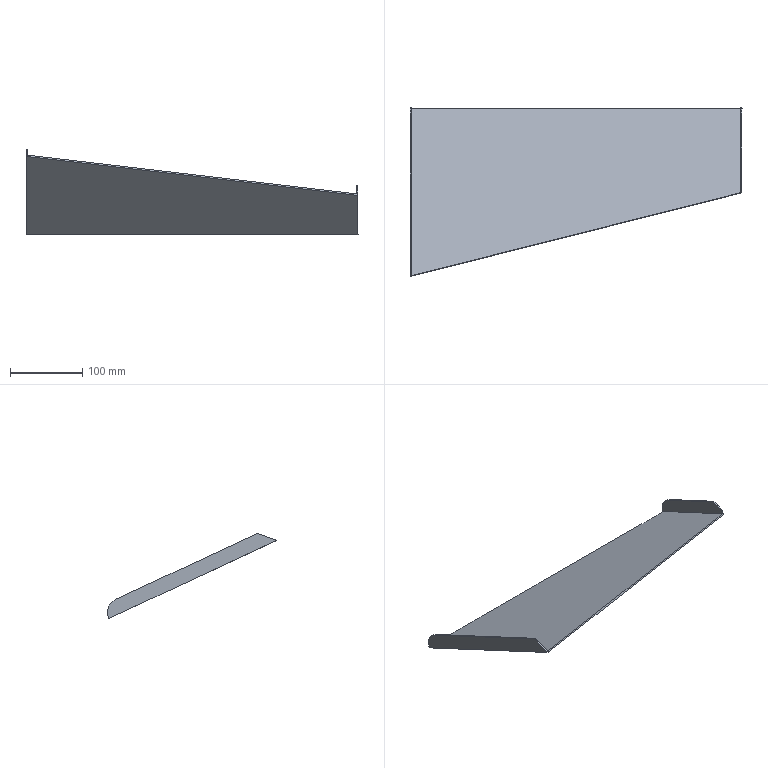Part | NX | features solid 2 | 1 solid | 16 faces | box 459.183 x 234.003 x 117.917 mm | volume 189236 mm3 | plane 13 | cylinder 2 | spline 1 | commonest cylinder face diameters 40 x2
STEP:
#1=CARTESIAN_POINT('',(244.183,710.326,-255.572));
#2=VERTEX_POINT('',#1);
#3=CARTESIAN_POINT('',(244.183,622.552,-214.642));
#4=VERTEX_POINT('',#3);
#5=CARTESIAN_POINT('',(244.183,728.452,-264.024));
#6=DIRECTION('',(0.,-0.9063,0.4226));
#7=VECTOR('',#6,1000.);
#8=LINE('',#5,#7);
#9=EDGE_CURVE('',#2,#4,#8,.T.);
#10=ORIENTED_EDGE('',*,*,#9,.F.);
#11=CARTESIAN_POINT('',(242.183,710.326,-255.572));
#12=VERTEX_POINT('',#11);
#13=CARTESIAN_POINT('',(214.183,710.326,-255.572));
#14=DIRECTION('',(-1.,0.,0.));
#15=VECTOR('',#14,1000.);
#16=LINE('',#13,#15);
#17=EDGE_CURVE('',#2,#12,#16,.T.);
#18=ORIENTED_EDGE('',*,*,#17,.T.);
#19=CARTESIAN_POINT('',(242.183,622.552,-214.642));
#20=VERTEX_POINT('',#19);
#21=CARTESIAN_POINT('',(242.183,728.452,-264.024));
#22=DIRECTION('',(0.,-0.9063,0.4226));
#23=VECTOR('',#22,1000.);
#24=LINE('',#21,#23);
#25=EDGE_CURVE('',#12,#20,#24,.T.);
#26=ORIENTED_EDGE('',*,*,#25,.T.);
#27=CARTESIAN_POINT('',(214.183,622.552,-214.642));
#28=DIRECTION('',(1.,0.,0.));
#29=VECTOR('',#28,1000.);
#30=LINE('',#27,#29);
#31=EDGE_CURVE('',#20,#4,#30,.T.);
#32=ORIENTED_EDGE('',*,*,#31,.T.);
#33=EDGE_LOOP('',(#10,#18,#26,#32));
#34=FACE_BOUND('',#33,.T.);
#35=CARTESIAN_POINT('',(214.183,728.452,-264.024));
#36=DIRECTION('',(0.,-0.4226,-0.9063));
#37=DIRECTION('',(0.,-0.9063,0.4226));
#38=AXIS2_PLACEMENT_3D('',#35,#36,#37);
#39=PLANE('',#38);
#40=ADVANCED_FACE('',(#34),#39,.F.);
#41=CARTESIAN_POINT('',(242.183,720.,-279.943));
#42=VERTEX_POINT('',#41);
#43=CARTESIAN_POINT('',(242.183,603.874,-225.793));
#44=VERTEX_POINT('',#43);
#45=CARTESIAN_POINT('',(242.183,417.055,-138.678));
#46=DIRECTION('',(0.,-0.9063,0.4226));
#47=VECTOR('',#46,1000.);
#48=LINE('',#45,#47);
#49=EDGE_CURVE('',#42,#44,#48,.T.);
#50=ORIENTED_EDGE('',*,*,#49,.T.);
#51=CARTESIAN_POINT('',(242.183,606.319,-220.55));
#52=VERTEX_POINT('',#51);
#53=CARTESIAN_POINT('',(242.183,606.319,-220.55));
#54=DIRECTION('',(0.,-0.4226,-0.9063));
#55=VECTOR('',#54,1000.);
#56=LINE('',#53,#55);
#57=EDGE_CURVE('',#44,#52,#56,.F.);
#58=ORIENTED_EDGE('',*,*,#57,.T.);
#59=CARTESIAN_POINT('',(242.183,686.904,-191.22));
#60=DIRECTION('',(0.,0.9397,0.342));
#61=VECTOR('',#60,1000.);
#62=LINE('',#59,#61);
#63=EDGE_CURVE('',#52,#20,#62,.T.);
#64=ORIENTED_EDGE('',*,*,#63,.T.);
#65=ORIENTED_EDGE('',*,*,#25,.F.);
#66=CARTESIAN_POINT('',(242.183,720.,-282.15));
#67=VERTEX_POINT('',#66);
#68=CARTESIAN_POINT('',(242.183,701.874,-273.698));
#69=DIRECTION('',(-1.,0.,0.));
#70=DIRECTION('',(0.,-1.,0.));
#71=AXIS2_PLACEMENT_3D('',#68,#69,#70);
#72=CIRCLE('',#71,20.);
#73=EDGE_CURVE('',#12,#67,#72,.T.);
#74=ORIENTED_EDGE('',*,*,#73,.T.);
#75=CARTESIAN_POINT('',(242.183,720.,-430.));
#76=DIRECTION('',(0.,0.,-1.));
#77=VECTOR('',#76,1000.);
#78=LINE('',#75,#77);
#79=EDGE_CURVE('',#42,#67,#78,.T.);
#80=ORIENTED_EDGE('',*,*,#79,.F.);
#81=EDGE_LOOP('',(#50,#58,#64,#65,#74,#80));
#82=FACE_BOUND('',#81,.T.);
#83=CARTESIAN_POINT('',(242.183,720.,-282.15));
#84=DIRECTION('',(-1.,0.,0.));
#85=DIRECTION('',(0.,-1.,0.));
#86=AXIS2_PLACEMENT_3D('',#83,#84,#85);
#87=PLANE('',#86);
#88=ADVANCED_FACE('',(#82),#87,.T.);
#89=ORIENTED_EDGE('',*,*,#63,.F.);
#90=CARTESIAN_POINT('',(244.183,607.058,-220.281));
#91=VERTEX_POINT('',#90);
#92=CARTESIAN_POINT('',(244.183,607.058,-220.281));
#93=CARTESIAN_POINT('',(243.516,606.812,-220.371));
#94=CARTESIAN_POINT('',(242.85,606.566,-220.461));
#95=CARTESIAN_POINT('',(242.183,606.319,-220.55));
#96=B_SPLINE_CURVE_WITH_KNOTS('',3,(#92,#93,#94,#95),.UNSPECIFIED.,.F.,.F.,(4,4),(0.1738,0.176),.UNSPECIFIED.);
#97=EDGE_CURVE('',#52,#91,#96,.F.);
#98=ORIENTED_EDGE('',*,*,#97,.T.);
#99=CARTESIAN_POINT('',(244.183,570.633,-233.539));
#100=DIRECTION('',(0.,-0.9397,-0.342));
#101=VECTOR('',#100,1000.);
#102=LINE('',#99,#101);
#103=EDGE_CURVE('',#4,#91,#102,.T.);
#104=ORIENTED_EDGE('',*,*,#103,.F.);
#105=ORIENTED_EDGE('',*,*,#31,.F.);
#106=EDGE_LOOP('',(#89,#98,#104,#105));
#107=FACE_BOUND('',#106,.T.);
#108=CARTESIAN_POINT('',(214.183,595.974,-224.316));
#109=DIRECTION('',(0.,-0.342,0.9397));
#110=DIRECTION('',(0.,-0.9397,-0.342));
#111=AXIS2_PLACEMENT_3D('',#108,#109,#110);
#112=PLANE('',#111);
#113=ADVANCED_FACE('',(#107),#112,.T.);
#114=CARTESIAN_POINT('',(244.183,603.533,-227.841));
#115=VERTEX_POINT('',#114);
#116=CARTESIAN_POINT('',(244.183,603.956,-226.934));
#117=DIRECTION('',(0.,-0.4226,-0.9063));
#118=VECTOR('',#117,1000.);
#119=LINE('',#116,#118);
#120=EDGE_CURVE('',#91,#115,#119,.T.);
#121=ORIENTED_EDGE('',*,*,#120,.T.);
#122=CARTESIAN_POINT('',(244.183,720.,-282.15));
#123=VERTEX_POINT('',#122);
#124=CARTESIAN_POINT('',(244.183,559.597,-207.353));
#125=DIRECTION('',(0.,-0.9063,0.4226));
#126=VECTOR('',#125,1000.);
#127=LINE('',#124,#126);
#128=EDGE_CURVE('',#123,#115,#127,.T.);
#129=ORIENTED_EDGE('',*,*,#128,.F.);
#130=CARTESIAN_POINT('',(244.183,701.874,-273.698));
#131=DIRECTION('',(1.,0.,0.));
#132=DIRECTION('',(0.,1.,0.));
#133=AXIS2_PLACEMENT_3D('',#130,#131,#132);
#134=CIRCLE('',#133,20.);
#135=EDGE_CURVE('',#123,#2,#134,.T.);
#136=ORIENTED_EDGE('',*,*,#135,.T.);
#137=ORIENTED_EDGE('',*,*,#9,.T.);
#138=ORIENTED_EDGE('',*,*,#103,.T.);
#139=EDGE_LOOP('',(#121,#129,#136,#137,#138));
#140=FACE_BOUND('',#139,.T.);
#141=CARTESIAN_POINT('',(244.183,560.442,-205.54));
#142=DIRECTION('',(1.,0.,0.));
#143=DIRECTION('',(0.,1.,0.));
#144=AXIS2_PLACEMENT_3D('',#141,#142,#143);
#145=PLANE('',#144);
#146=ADVANCED_FACE('',(#140),#145,.T.);
#147=ORIENTED_EDGE('',*,*,#135,.F.);
#148=CARTESIAN_POINT('',(188.564,720.,-282.15));
#149=DIRECTION('',(-1.,0.,0.));
#150=VECTOR('',#149,1000.);
#151=LINE('',#148,#150);
#152=EDGE_CURVE('',#123,#67,#151,.T.);
#153=ORIENTED_EDGE('',*,*,#152,.T.);
#154=ORIENTED_EDGE('',*,*,#73,.F.);
#155=ORIENTED_EDGE('',*,*,#17,.F.);
#156=EDGE_LOOP('',(#147,#153,#154,#155));
#157=FACE_BOUND('',#156,.T.);
#158=CARTESIAN_POINT('',(214.183,701.874,-273.698));
#159=DIRECTION('',(-1.,0.,0.));
#160=DIRECTION('',(0.,-1.,0.));
#161=AXIS2_PLACEMENT_3D('',#158,#159,#160);
#162=CYLINDRICAL_SURFACE('',#161,20.);
#163=ADVANCED_FACE('',(#157),#162,.T.);
#164=CARTESIAN_POINT('',(-213.,488.372,-174.14));
#165=VERTEX_POINT('',#164);
#166=CARTESIAN_POINT('',(-213.,488.372,-174.14));
#167=CARTESIAN_POINT('',(-174.889,497.929,-178.597));
#168=CARTESIAN_POINT('',(-98.706,517.168,-187.568));
#169=CARTESIAN_POINT('',(53.68,555.581,-205.48));
#170=CARTESIAN_POINT('',(167.988,584.333,-218.888));
#171=CARTESIAN_POINT('',(244.183,603.533,-227.841));
#172=B_SPLINE_CURVE_WITH_KNOTS('',3,(#166,#167,#168,#169,#170,#171),.UNSPECIFIED.,.F.,.F.,(4,1,1,4),(0.,0.1186,0.2373,0.4745),.UNSPECIFIED.);
#173=EDGE_CURVE('',#165,#115,#172,.T.);
#174=ORIENTED_EDGE('',*,*,#173,.F.);
#175=CARTESIAN_POINT('',(-213.,487.871,-173.907));
#176=VERTEX_POINT('',#175);
#177=CARTESIAN_POINT('',(-213.,487.871,-173.907));
#178=DIRECTION('',(0.,0.9063,-0.4226));
#179=VECTOR('',#178,1000.);
#180=LINE('',#177,#179);
#181=EDGE_CURVE('',#176,#165,#180,.T.);
#182=ORIENTED_EDGE('',*,*,#181,.F.);
#183=CARTESIAN_POINT('',(-215.,487.871,-173.907));
#184=VERTEX_POINT('',#183);
#185=CARTESIAN_POINT('',(-215.,487.871,-173.907));
#186=DIRECTION('',(1.,0.,0.));
#187=VECTOR('',#186,1000.);
#188=LINE('',#185,#187);
#189=EDGE_CURVE('',#184,#176,#188,.T.);
#190=ORIENTED_EDGE('',*,*,#189,.F.);
#191=CARTESIAN_POINT('',(-215.,720.,-282.15));
#192=VERTEX_POINT('',#191);
#193=CARTESIAN_POINT('',(-215.,416.21,-140.491));
#194=DIRECTION('',(0.,0.9063,-0.4226));
#195=VECTOR('',#194,1000.);
#196=LINE('',#193,#195);
#197=EDGE_CURVE('',#184,#192,#196,.T.);
#198=ORIENTED_EDGE('',*,*,#197,.T.);
#199=CARTESIAN_POINT('',(-213.,720.,-282.15));
#200=VERTEX_POINT('',#199);
#201=CARTESIAN_POINT('',(-215.,720.,-282.15));
#202=DIRECTION('',(1.,0.,0.));
#203=VECTOR('',#202,1000.);
#204=LINE('',#201,#203);
#205=EDGE_CURVE('',#192,#200,#204,.T.);
#206=ORIENTED_EDGE('',*,*,#205,.T.);
#207=CARTESIAN_POINT('',(188.564,720.,-282.15));
#208=DIRECTION('',(-1.,0.,0.));
#209=VECTOR('',#208,1000.);
#210=LINE('',#207,#209);
#211=EDGE_CURVE('',#67,#200,#210,.T.);
#212=ORIENTED_EDGE('',*,*,#211,.F.);
#213=ORIENTED_EDGE('',*,*,#152,.F.);
#214=ORIENTED_EDGE('',*,*,#128,.T.);
#215=EDGE_LOOP('',(#174,#182,#190,#198,#206,#212,#213,#214));
#216=FACE_BOUND('',#215,.T.);
#217=CARTESIAN_POINT('',(-353.018,416.21,-140.491));
#218=DIRECTION('',(0.,0.4226,0.9063));
#219=DIRECTION('',(1.,0.,0.));
#220=AXIS2_PLACEMENT_3D('',#217,#218,#219);
#221=PLANE('',#220);
#222=ADVANCED_FACE('',(#216),#221,.F.);
#223=CARTESIAN_POINT('',(221.376,598.631,-223.348));
#224=VERTEX_POINT('',#223);
#225=CARTESIAN_POINT('',(-677.72,244.443,-58.187));
#226=CARTESIAN_POINT('',(-660.306,267.421,-68.902));
#227=CARTESIAN_POINT('',(-639.328,288.979,-78.955));
#228=CARTESIAN_POINT('',(-618.744,310.134,-88.819));
#229=CARTESIAN_POINT('',(-595.443,329.078,-97.653));
#230=CARTESIAN_POINT('',(-550.727,365.432,-114.606));
#231=CARTESIAN_POINT('',(-494.661,394.945,-128.368));
#232=CARTESIAN_POINT('',(-442.667,422.315,-141.131));
#233=CARTESIAN_POINT('',(-382.139,443.144,-150.843));
#234=CARTESIAN_POINT('',(-352.965,453.184,-155.525));
#235=CARTESIAN_POINT('',(-323.451,461.202,-159.264));
#236=CARTESIAN_POINT('',(-311.851,464.353,-160.733));
#237=CARTESIAN_POINT('',(-289.398,470.048,-163.389));
#238=CARTESIAN_POINT('',(-278.105,472.912,-164.724));
#239=CARTESIAN_POINT('',(-263.795,476.502,-166.398));
#240=CARTESIAN_POINT('',(-257.293,478.133,-167.159));
#241=CARTESIAN_POINT('',(-233.907,483.982,-169.886));
#242=CARTESIAN_POINT('',(-218.807,487.759,-171.647));
#243=CARTESIAN_POINT('',(-204.022,491.47,-173.378));
#244=CARTESIAN_POINT('',(-178.964,497.761,-176.312));
#245=CARTESIAN_POINT('',(-144.274,506.511,-180.392));
#246=CARTESIAN_POINT('',(-27.735,535.905,-194.099));
#247=CARTESIAN_POINT('',(-24.798,536.645,-194.444));
#248=CARTESIAN_POINT('',(13.703,546.346,-198.967));
#249=CARTESIAN_POINT('',(94.693,566.731,-208.473));
#250=CARTESIAN_POINT('',(173.185,586.488,-217.686));
#251=CARTESIAN_POINT('',(214.183,596.819,-222.503));
#252=CARTESIAN_POINT('',(229.183,600.599,-224.266));
#253=CARTESIAN_POINT('',(244.183,604.378,-226.028));
#254=B_SPLINE_CURVE_WITH_KNOTS('',2,(#225,#226,#227,#228,#229,#230,#231,#232,#233,#234,#235,#236,#237,#238,#239,#240,#241,#242,#243,#244,#245,#246,#247,#248,#249,#250,#251,#252,#253),.UNSPECIFIED.,.F.,.F.,(3,2,2,2,2,2,2,2,2,2,2,2,2,2,3),(0.,0.0625,0.125,0.25,0.375,0.4375,0.4732,0.5,0.5312,0.5625,0.625,0.75,0.875,1.,1.046),.PIECEWISE_BEZIER_KNOTS.);
#255=EDGE_CURVE('',#224,#44,#254,.T.);
#256=ORIENTED_EDGE('',*,*,#255,.F.);
#257=CARTESIAN_POINT('',(-215.,488.716,-172.094));
#258=VERTEX_POINT('',#257);
#259=CARTESIAN_POINT('',(-215.,488.716,-172.094));
#260=CARTESIAN_POINT('',(-142.246,506.955,-180.599));
#261=CARTESIAN_POINT('',(3.163,543.756,-197.76));
#262=CARTESIAN_POINT('',(148.649,580.305,-214.803));
#263=CARTESIAN_POINT('',(221.376,598.631,-223.348));
#264=B_SPLINE_CURVE_WITH_KNOTS('',3,(#259,#260,#261,#262,#263),.UNSPECIFIED.,.F.,.F.,(4,1,4),(0.,0.2265,0.4529),.UNSPECIFIED.);
#265=EDGE_CURVE('',#258,#224,#264,.T.);
#266=ORIENTED_EDGE('',*,*,#265,.F.);
#267=CARTESIAN_POINT('',(-215.,488.294,-173.));
#268=DIRECTION('',(0.,-0.4226,-0.9063));
#269=VECTOR('',#268,1000.);
#270=LINE('',#267,#269);
#271=EDGE_CURVE('',#258,#184,#270,.T.);
#272=ORIENTED_EDGE('',*,*,#271,.T.);
#273=CARTESIAN_POINT('',(-213.,488.606,-173.639));
#274=VERTEX_POINT('',#273);
#275=CARTESIAN_POINT('',(-215.,487.871,-173.907));
#276=CARTESIAN_POINT('',(-214.333,488.116,-173.817));
#277=CARTESIAN_POINT('',(-213.667,488.361,-173.728));
#278=CARTESIAN_POINT('',(-213.,488.606,-173.639));
#279=B_SPLINE_CURVE_WITH_KNOTS('',3,(#275,#276,#277,#278),.UNSPECIFIED.,.F.,.F.,(4,4),(0.,0.002148),.UNSPECIFIED.);
#280=EDGE_CURVE('',#184,#274,#279,.T.);
#281=ORIENTED_EDGE('',*,*,#280,.T.);
#282=CARTESIAN_POINT('',(-213.,489.218,-172.328));
#283=DIRECTION('',(0.,-0.4226,-0.9063));
#284=VECTOR('',#283,1000.);
#285=LINE('',#282,#284);
#286=EDGE_CURVE('',#274,#165,#285,.T.);
#287=ORIENTED_EDGE('',*,*,#286,.T.);
#288=ORIENTED_EDGE('',*,*,#173,.T.);
#289=ORIENTED_EDGE('',*,*,#120,.F.);
#290=ORIENTED_EDGE('',*,*,#97,.F.);
#291=ORIENTED_EDGE('',*,*,#57,.F.);
#292=EDGE_LOOP('',(#256,#266,#272,#281,#287,#288,#289,#290,#291));
#293=FACE_BOUND('',#292,.T.);
#294=CARTESIAN_POINT('',(-215.,491.417,-166.302));
#295=CARTESIAN_POINT('',(-215.,487.871,-173.907));
#296=CARTESIAN_POINT('',(-213.771,491.725,-166.445));
#297=CARTESIAN_POINT('',(-213.771,488.179,-174.05));
#298=CARTESIAN_POINT('',(-211.321,492.34,-166.732));
#299=CARTESIAN_POINT('',(-211.321,488.794,-174.337));
#300=CARTESIAN_POINT('',(-208.246,493.111,-167.092));
#301=CARTESIAN_POINT('',(-208.246,489.565,-174.697));
#302=CARTESIAN_POINT('',(-205.832,493.717,-167.374));
#303=CARTESIAN_POINT('',(-205.832,490.171,-174.979));
#304=CARTESIAN_POINT('',(-203.913,494.199,-167.599));
#305=CARTESIAN_POINT('',(-203.913,490.653,-175.204));
#306=CARTESIAN_POINT('',(-202.454,494.565,-167.77));
#307=CARTESIAN_POINT('',(-202.454,491.019,-175.374));
#308=CARTESIAN_POINT('',(-200.317,495.102,-168.02));
#309=CARTESIAN_POINT('',(-200.317,491.555,-175.625));
#310=CARTESIAN_POINT('',(-197.658,495.77,-168.331));
#311=CARTESIAN_POINT('',(-197.658,492.223,-175.936));
#312=CARTESIAN_POINT('',(-193.272,496.872,-168.845));
#313=CARTESIAN_POINT('',(-193.272,493.326,-176.45));
#314=CARTESIAN_POINT('',(-187.616,498.294,-169.508));
#315=CARTESIAN_POINT('',(-187.616,494.747,-177.113));
#316=CARTESIAN_POINT('',(-180.53,500.076,-170.34));
#317=CARTESIAN_POINT('',(-180.53,496.53,-177.944));
#318=CARTESIAN_POINT('',(-173.151,501.934,-171.206));
#319=CARTESIAN_POINT('',(-173.151,498.388,-178.811));
#320=CARTESIAN_POINT('',(-166.755,503.545,-171.957));
#321=CARTESIAN_POINT('',(-166.755,499.999,-179.562));
#322=CARTESIAN_POINT('',(-161.492,504.871,-172.575));
#323=CARTESIAN_POINT('',(-161.492,501.325,-180.18));
#324=CARTESIAN_POINT('',(-157.47,505.885,-173.048));
#325=CARTESIAN_POINT('',(-157.47,502.338,-180.653));
#326=CARTESIAN_POINT('',(-154.057,506.745,-173.449));
#327=CARTESIAN_POINT('',(-154.057,503.199,-181.054));
#328=CARTESIAN_POINT('',(-151.291,507.442,-173.774));
#329=CARTESIAN_POINT('',(-151.291,503.896,-181.379));
#330=CARTESIAN_POINT('',(-149.195,507.971,-174.021));
#331=CARTESIAN_POINT('',(-149.195,504.425,-181.626));
#332=CARTESIAN_POINT('',(-147.441,508.413,-174.227));
#333=CARTESIAN_POINT('',(-147.441,504.867,-181.832));
#334=CARTESIAN_POINT('',(-146.012,508.774,-174.395));
#335=CARTESIAN_POINT('',(-146.012,505.227,-182.));
#336=CARTESIAN_POINT('',(-145.153,508.99,-174.496));
#337=CARTESIAN_POINT('',(-145.153,505.444,-182.101));
#338=CARTESIAN_POINT('',(-144.522,509.149,-174.57));
#339=CARTESIAN_POINT('',(-144.522,505.603,-182.175));
#340=CARTESIAN_POINT('',(-144.305,509.204,-174.596));
#341=CARTESIAN_POINT('',(-144.305,505.658,-182.201));
#342=CARTESIAN_POINT('',(-143.977,509.287,-174.635));
#343=CARTESIAN_POINT('',(-143.977,505.741,-182.239));
#344=CARTESIAN_POINT('',(-143.469,509.415,-174.694));
#345=CARTESIAN_POINT('',(-143.469,505.869,-182.299));
#346=CARTESIAN_POINT('',(-142.712,509.606,-174.783));
#347=CARTESIAN_POINT('',(-142.712,506.06,-182.388));
#348=CARTESIAN_POINT('',(-141.525,509.905,-174.923));
#349=CARTESIAN_POINT('',(-141.525,506.359,-182.528));
#350=CARTESIAN_POINT('',(-140.043,510.279,-175.097));
#351=CARTESIAN_POINT('',(-140.043,506.733,-182.702));
#352=CARTESIAN_POINT('',(-136.518,511.168,-175.512));
#353=CARTESIAN_POINT('',(-136.518,507.622,-183.117));
#354=CARTESIAN_POINT('',(-131.33,512.477,-176.122));
#355=CARTESIAN_POINT('',(-131.33,508.931,-183.727));
#356=CARTESIAN_POINT('',(-124.631,514.166,-176.91));
#357=CARTESIAN_POINT('',(-124.631,510.62,-184.515));
#358=CARTESIAN_POINT('',(-118.15,515.801,-177.672));
#359=CARTESIAN_POINT('',(-118.15,512.255,-185.277));
#360=CARTESIAN_POINT('',(-109.797,517.908,-178.655));
#361=CARTESIAN_POINT('',(-109.797,514.362,-186.259));
#362=CARTESIAN_POINT('',(-99.9,520.404,-179.819));
#363=CARTESIAN_POINT('',(-99.9,516.858,-187.424));
#364=CARTESIAN_POINT('',(-88.892,523.181,-181.113));
#365=CARTESIAN_POINT('',(-88.892,519.635,-188.718));
#366=CARTESIAN_POINT('',(-78.753,525.738,-182.306));
#367=CARTESIAN_POINT('',(-78.753,522.192,-189.911));
#368=CARTESIAN_POINT('',(-66.394,528.855,-183.759));
#369=CARTESIAN_POINT('',(-66.394,525.309,-191.364));
#370=CARTESIAN_POINT('',(-53.117,532.204,-185.321));
#371=CARTESIAN_POINT('',(-53.117,528.658,-192.926));
#372=CARTESIAN_POINT('',(-42.738,534.822,-186.542));
#373=CARTESIAN_POINT('',(-42.738,531.276,-194.147));
#374=CARTESIAN_POINT('',(-36.173,536.478,-187.314));
#375=CARTESIAN_POINT('',(-36.173,532.932,-194.919));
#376=CARTESIAN_POINT('',(-32.118,537.501,-187.791));
#377=CARTESIAN_POINT('',(-32.118,533.954,-195.396));
#378=CARTESIAN_POINT('',(-28.932,538.304,-188.165));
#379=CARTESIAN_POINT('',(-28.932,534.758,-195.77));
#380=CARTESIAN_POINT('',(-27.001,538.791,-188.392));
#381=CARTESIAN_POINT('',(-27.001,535.245,-195.997));
#382=CARTESIAN_POINT('',(-25.891,539.071,-188.523));
#383=CARTESIAN_POINT('',(-25.891,535.525,-196.128));
#384=CARTESIAN_POINT('',(-25.379,539.2,-188.583));
#385=CARTESIAN_POINT('',(-25.379,535.654,-196.188));
#386=CARTESIAN_POINT('',(-25.114,539.267,-188.614));
#387=CARTESIAN_POINT('',(-25.114,535.72,-196.219));
#388=CARTESIAN_POINT('',(-24.992,539.297,-188.629));
#389=CARTESIAN_POINT('',(-24.992,535.751,-196.234));
#390=CARTESIAN_POINT('',(-24.909,539.318,-188.638));
#391=CARTESIAN_POINT('',(-24.909,535.772,-196.243));
#392=CARTESIAN_POINT('',(-24.867,539.329,-188.643));
#393=CARTESIAN_POINT('',(-24.867,535.783,-196.248));
#394=CARTESIAN_POINT('',(-24.804,539.345,-188.651));
#395=CARTESIAN_POINT('',(-24.804,535.799,-196.256));
#396=CARTESIAN_POINT('',(-24.861,539.331,-188.644));
#397=CARTESIAN_POINT('',(-24.861,535.784,-196.249));
#398=CARTESIAN_POINT('',(-24.468,539.429,-188.69));
#399=CARTESIAN_POINT('',(-24.468,535.883,-196.295));
#400=CARTESIAN_POINT('',(-24.1,539.522,-188.734));
#401=CARTESIAN_POINT('',(-24.1,535.976,-196.338));
#402=CARTESIAN_POINT('',(-23.377,539.704,-188.818));
#403=CARTESIAN_POINT('',(-23.377,536.158,-196.423));
#404=CARTESIAN_POINT('',(-22.37,539.958,-188.937));
#405=CARTESIAN_POINT('',(-22.37,536.412,-196.542));
#406=CARTESIAN_POINT('',(-20.71,540.376,-189.132));
#407=CARTESIAN_POINT('',(-20.71,536.83,-196.737));
#408=CARTESIAN_POINT('',(-18.592,540.91,-189.381));
#409=CARTESIAN_POINT('',(-18.592,537.364,-196.985));
#410=CARTESIAN_POINT('',(-15.966,541.571,-189.689));
#411=CARTESIAN_POINT('',(-15.966,538.025,-197.294));
#412=CARTESIAN_POINT('',(-12.357,542.48,-190.113));
#413=CARTESIAN_POINT('',(-12.357,538.934,-197.718));
#414=CARTESIAN_POINT('',(-7.643,543.668,-190.667));
#415=CARTESIAN_POINT('',(-7.643,540.122,-198.272));
#416=CARTESIAN_POINT('',(-1.661,545.175,-191.369));
#417=CARTESIAN_POINT('',(-1.661,541.628,-198.974));
#418=CARTESIAN_POINT('',(4.647,546.763,-192.11));
#419=CARTESIAN_POINT('',(4.647,543.217,-199.715));
#420=CARTESIAN_POINT('',(13.49,548.99,-193.148));
#421=CARTESIAN_POINT('',(13.49,545.444,-200.753));
#422=CARTESIAN_POINT('',(25.356,551.978,-194.542));
#423=CARTESIAN_POINT('',(25.356,548.432,-202.146));
#424=CARTESIAN_POINT('',(40.897,555.89,-196.366));
#425=CARTESIAN_POINT('',(40.897,552.344,-203.971));
#426=CARTESIAN_POINT('',(54.93,559.423,-198.013));
#427=CARTESIAN_POINT('',(54.93,555.877,-205.618));
#428=CARTESIAN_POINT('',(66.808,562.413,-199.408));
#429=CARTESIAN_POINT('',(66.808,558.867,-207.013));
#430=CARTESIAN_POINT('',(76.04,564.737,-200.491));
#431=CARTESIAN_POINT('',(76.04,561.191,-208.096));
#432=CARTESIAN_POINT('',(84.008,566.743,-201.427));
#433=CARTESIAN_POINT('',(84.008,563.197,-209.031));
#434=CARTESIAN_POINT('',(90.536,568.386,-202.193));
#435=CARTESIAN_POINT('',(90.536,564.84,-209.798));
#436=CARTESIAN_POINT('',(97.206,570.065,-202.976));
#437=CARTESIAN_POINT('',(97.206,566.519,-210.581));
#438=CARTESIAN_POINT('',(105.077,572.046,-203.9));
#439=CARTESIAN_POINT('',(105.077,568.5,-211.504));
#440=CARTESIAN_POINT('',(117.449,575.16,-205.352));
#441=CARTESIAN_POINT('',(117.449,571.614,-212.957));
#442=CARTESIAN_POINT('',(132.141,578.859,-207.076));
#443=CARTESIAN_POINT('',(132.141,575.312,-214.681));
#444=CARTESIAN_POINT('',(148.648,583.014,-209.014));
#445=CARTESIAN_POINT('',(148.648,579.468,-216.619));
#446=CARTESIAN_POINT('',(164.001,586.88,-210.817));
#447=CARTESIAN_POINT('',(164.001,583.334,-218.422));
#448=CARTESIAN_POINT('',(178.208,590.458,-212.485));
#449=CARTESIAN_POINT('',(178.208,586.911,-220.09));
#450=CARTESIAN_POINT('',(191.269,593.747,-214.019));
#451=CARTESIAN_POINT('',(191.269,590.201,-221.624));
#452=CARTESIAN_POINT('',(201.192,596.247,-215.185));
#453=CARTESIAN_POINT('',(201.192,592.7,-222.789));
#454=CARTESIAN_POINT('',(208.567,598.105,-216.051));
#455=CARTESIAN_POINT('',(208.567,594.558,-223.656));
#456=CARTESIAN_POINT('',(213.784,599.419,-216.664));
#457=CARTESIAN_POINT('',(213.784,595.873,-224.269));
#458=CARTESIAN_POINT('',(218.819,600.688,-217.255));
#459=CARTESIAN_POINT('',(218.819,597.142,-224.86));
#460=CARTESIAN_POINT('',(228.978,603.248,-218.449));
#461=CARTESIAN_POINT('',(228.978,599.702,-226.054));
#462=CARTESIAN_POINT('',(237.421,605.375,-219.441));
#463=CARTESIAN_POINT('',(237.421,601.829,-227.046));
#464=CARTESIAN_POINT('',(244.183,607.079,-220.236));
#465=CARTESIAN_POINT('',(244.183,603.533,-227.841));
#466=B_SPLINE_SURFACE_WITH_KNOTS('',3,1,((#294,#295),(#296,#297),(#298,#299),(#300,#301),(#302,#303),(#304,#305),(#306,#307),(#308,#309),(#310,#311),(#312,#313),(#314,#315),(#316,#317),(#318,#319),(#320,#321),(#322,#323),(#324,#325),(#326,#327),(#328,#329),(#330,#331),(#332,#333),(#334,#335),(#336,#337),(#338,#339),(#340,#341),(#342,#343),(#344,#345),(#346,#347),(#348,#349),(#350,#351),(#352,#353),(#354,#355),(#356,#357),(#358,#359),(#360,#361),(#362,#363),(#364,#365),(#366,#367),(#368,#369),(#370,#371),(#372,#373),(#374,#375),(#376,#377),(#378,#379),(#380,#381),(#382,#383),(#384,#385),(#386,#387),(#388,#389),(#390,#391),(#392,#393),(#394,#395),(#396,#397),(#398,#399),(#400,#401),(#402,#403),(#404,#405),(#406,#407),(#408,#409),(#410,#411),(#412,#413),(#414,#415),(#416,#417),(#418,#419),(#420,#421),(#422,#423),(#424,#425),(#426,#427),(#428,#429),(#430,#431),(#432,#433),(#434,#435),(#436,#437),(#438,#439),(#440,#441),(#442,#443),(#444,#445),(#446,#447),(#448,#449),(#450,#451),(#452,#453),(#454,#455),(#456,#457),(#458,#459),(#460,#461),(#462,#463),(#464,#465)),.SURF_OF_LINEAR_EXTRUSION.,.F.,.F.,.F.,(4,1,1,1,1,1,1,1,1,1,1,1,1,1,1,1,1,1,1,1,1,1,1,1,1,1,1,1,1,1,1,1,1,1,1,1,1,1,1,1,1,1,1,1,1,1,1,1,1,1,1,1,1,1,1,1,1,1,1,1,1,1,1,1,1,1,1,1,1,1,1,1,1,1,1,1,1,1,1,1,1,1,1,4),(2,2),(0.5509,0.5548,0.5587,0.5606,0.5625,0.5645,0.5664,0.5703,0.5741,0.5819,0.5896,0.5973,0.6051,0.6089,0.6128,0.6167,0.6186,0.6205,0.6225,0.6234,0.6244,0.6249,0.625,0.6251,0.6254,0.6258,0.6263,0.6273,0.6283,0.6321,0.636,0.6399,0.6437,0.6514,0.6592,0.6669,0.6746,0.6901,0.7056,0.7133,0.721,0.7288,0.7365,0.7404,0.7442,0.7462,0.7471,0.7481,0.7491,0.7495,0.75,0.7505,0.751,0.752,0.7539,0.7558,0.7597,0.7635,0.7674,0.7751,0.7829,0.7906,0.7983,0.8138,0.8293,0.8447,0.8525,0.8602,0.8679,0.8718,0.8756,0.8834,0.8911,0.9066,0.922,0.9375,0.953,0.9684,0.9839,0.9916,0.9993,1.007,1.015,1.046),(0.,1.),.UNSPECIFIED.);
#467=ADVANCED_FACE('',(#293),#466,.F.);
#468=ORIENTED_EDGE('',*,*,#265,.T.);
#469=ORIENTED_EDGE('',*,*,#255,.T.);
#470=ORIENTED_EDGE('',*,*,#49,.F.);
#471=CARTESIAN_POINT('',(-213.,720.,-279.943));
#472=VERTEX_POINT('',#471);
#473=CARTESIAN_POINT('',(188.564,720.,-279.943));
#474=DIRECTION('',(-1.,0.,0.));
#475=VECTOR('',#474,1000.);
#476=LINE('',#473,#475);
#477=EDGE_CURVE('',#42,#472,#476,.T.);
#478=ORIENTED_EDGE('',*,*,#477,.T.);
#479=CARTESIAN_POINT('',(-213.,490.529,-172.939));
#480=VERTEX_POINT('',#479);
#481=CARTESIAN_POINT('',(-213.,417.055,-138.678));
#482=DIRECTION('',(0.,0.9063,-0.4226));
#483=VECTOR('',#482,1000.);
#484=LINE('',#481,#483);
#485=EDGE_CURVE('',#480,#472,#484,.T.);
#486=ORIENTED_EDGE('',*,*,#485,.F.);
#487=CARTESIAN_POINT('',(-215.,490.529,-172.939));
#488=VERTEX_POINT('',#487);
#489=CARTESIAN_POINT('',(-353.018,490.529,-172.939));
#490=DIRECTION('',(-1.,0.,0.));
#491=VECTOR('',#490,1000.);
#492=LINE('',#489,#491);
#493=EDGE_CURVE('',#488,#480,#492,.F.);
#494=ORIENTED_EDGE('',*,*,#493,.F.);
#495=CARTESIAN_POINT('',(-215.,417.055,-138.678));
#496=DIRECTION('',(0.,0.9063,-0.4226));
#497=VECTOR('',#496,1000.);
#498=LINE('',#495,#497);
#499=EDGE_CURVE('',#258,#488,#498,.T.);
#500=ORIENTED_EDGE('',*,*,#499,.F.);
#501=EDGE_LOOP('',(#468,#469,#470,#478,#486,#494,#500));
#502=FACE_BOUND('',#501,.T.);
#503=CARTESIAN_POINT('',(-353.018,417.055,-138.678));
#504=DIRECTION('',(0.,0.4226,0.9063));
#505=DIRECTION('',(1.,0.,0.));
#506=AXIS2_PLACEMENT_3D('',#503,#504,#505);
#507=PLANE('',#506);
#508=ADVANCED_FACE('',(#502),#507,.T.);
#509=ORIENTED_EDGE('',*,*,#211,.T.);
#510=CARTESIAN_POINT('',(-213.,720.,-430.));
#511=DIRECTION('',(0.,0.,1.));
#512=VECTOR('',#511,1000.);
#513=LINE('',#510,#512);
#514=EDGE_CURVE('',#200,#472,#513,.T.);
#515=ORIENTED_EDGE('',*,*,#514,.T.);
#516=ORIENTED_EDGE('',*,*,#477,.F.);
#517=ORIENTED_EDGE('',*,*,#79,.T.);
#518=EDGE_LOOP('',(#509,#515,#516,#517));
#519=FACE_BOUND('',#518,.T.);
#520=CARTESIAN_POINT('',(188.564,720.,-430.));
#521=DIRECTION('',(0.,-1.,0.));
#522=DIRECTION('',(-1.,0.,0.));
#523=AXIS2_PLACEMENT_3D('',#520,#521,#522);
#524=PLANE('',#523);
#525=ADVANCED_FACE('',(#519),#524,.F.);
#526=ORIENTED_EDGE('',*,*,#499,.T.);
#527=CARTESIAN_POINT('',(-215.,514.45,-164.233));
#528=VERTEX_POINT('',#527);
#529=CARTESIAN_POINT('',(-215.,514.45,-164.233));
#530=DIRECTION('',(0.,-0.9397,-0.342));
#531=VECTOR('',#530,1000.);
#532=LINE('',#529,#531);
#533=EDGE_CURVE('',#488,#528,#532,.F.);
#534=ORIENTED_EDGE('',*,*,#533,.T.);
#535=CARTESIAN_POINT('',(-215.,710.326,-255.572));
#536=VERTEX_POINT('',#535);
#537=CARTESIAN_POINT('',(-215.,496.323,-155.78));
#538=DIRECTION('',(0.,0.9063,-0.4226));
#539=VECTOR('',#538,1000.);
#540=LINE('',#537,#539);
#541=EDGE_CURVE('',#528,#536,#540,.T.);
#542=ORIENTED_EDGE('',*,*,#541,.T.);
#543=CARTESIAN_POINT('',(-215.,701.874,-273.698));
#544=DIRECTION('',(1.,0.,0.));
#545=DIRECTION('',(0.,0.,-1.));
#546=AXIS2_PLACEMENT_3D('',#543,#544,#545);
#547=CIRCLE('',#546,20.);
#548=EDGE_CURVE('',#536,#192,#547,.F.);
#549=ORIENTED_EDGE('',*,*,#548,.T.);
#550=ORIENTED_EDGE('',*,*,#197,.F.);
#551=ORIENTED_EDGE('',*,*,#271,.F.);
#552=EDGE_LOOP('',(#526,#534,#542,#549,#550,#551));
#553=FACE_BOUND('',#552,.T.);
#554=CARTESIAN_POINT('',(-215.,477.364,-105.));
#555=DIRECTION('',(1.,0.,0.));
#556=DIRECTION('',(0.,0.,-1.));
#557=AXIS2_PLACEMENT_3D('',#554,#555,#556);
#558=PLANE('',#557);
#559=ADVANCED_FACE('',(#553),#558,.F.);
#560=ORIENTED_EDGE('',*,*,#548,.F.);
#561=CARTESIAN_POINT('',(-213.,710.326,-255.572));
#562=VERTEX_POINT('',#561);
#563=CARTESIAN_POINT('',(-215.,710.326,-255.572));
#564=DIRECTION('',(1.,0.,0.));
#565=VECTOR('',#564,1000.);
#566=LINE('',#563,#565);
#567=EDGE_CURVE('',#562,#536,#566,.F.);
#568=ORIENTED_EDGE('',*,*,#567,.F.);
#569=CARTESIAN_POINT('',(-213.,701.874,-273.698));
#570=DIRECTION('',(1.,0.,0.));
#571=DIRECTION('',(0.,0.,-1.));
#572=AXIS2_PLACEMENT_3D('',#569,#570,#571);
#573=CIRCLE('',#572,20.);
#574=EDGE_CURVE('',#200,#562,#573,.T.);
#575=ORIENTED_EDGE('',*,*,#574,.F.);
#576=ORIENTED_EDGE('',*,*,#205,.F.);
#577=EDGE_LOOP('',(#560,#568,#575,#576));
#578=FACE_BOUND('',#577,.T.);
#579=CARTESIAN_POINT('',(-215.,701.874,-273.698));
#580=DIRECTION('',(-1.,0.,0.));
#581=DIRECTION('',(0.,0.,1.));
#582=AXIS2_PLACEMENT_3D('',#579,#580,#581);
#583=CYLINDRICAL_SURFACE('',#582,20.);
#584=ADVANCED_FACE('',(#578),#583,.T.);
#585=ORIENTED_EDGE('',*,*,#533,.F.);
#586=ORIENTED_EDGE('',*,*,#493,.T.);
#587=CARTESIAN_POINT('',(-213.,514.45,-164.233));
#588=VERTEX_POINT('',#587);
#589=CARTESIAN_POINT('',(-213.,487.871,-173.907));
#590=DIRECTION('',(0.,0.9397,0.342));
#591=VECTOR('',#590,1000.);
#592=LINE('',#589,#591);
#593=EDGE_CURVE('',#588,#480,#592,.F.);
#594=ORIENTED_EDGE('',*,*,#593,.F.);
#595=CARTESIAN_POINT('',(-215.,514.45,-164.233));
#596=DIRECTION('',(-1.,0.,0.));
#597=VECTOR('',#596,1000.);
#598=LINE('',#595,#597);
#599=EDGE_CURVE('',#528,#588,#598,.F.);
#600=ORIENTED_EDGE('',*,*,#599,.F.);
#601=EDGE_LOOP('',(#585,#586,#594,#600));
#602=FACE_BOUND('',#601,.T.);
#603=CARTESIAN_POINT('',(-215.,514.45,-164.233));
#604=DIRECTION('',(0.,0.342,-0.9397));
#605=DIRECTION('',(0.,0.9397,0.342));
#606=AXIS2_PLACEMENT_3D('',#603,#604,#605);
#607=PLANE('',#606);
#608=ADVANCED_FACE('',(#602),#607,.F.);
#609=ORIENTED_EDGE('',*,*,#593,.T.);
#610=ORIENTED_EDGE('',*,*,#485,.T.);
#611=ORIENTED_EDGE('',*,*,#514,.F.);
#612=ORIENTED_EDGE('',*,*,#574,.T.);
#613=CARTESIAN_POINT('',(-213.,496.323,-155.78));
#614=DIRECTION('',(0.,0.9063,-0.4226));
#615=VECTOR('',#614,1000.);
#616=LINE('',#613,#615);
#617=EDGE_CURVE('',#588,#562,#616,.T.);
#618=ORIENTED_EDGE('',*,*,#617,.F.);
#619=EDGE_LOOP('',(#609,#610,#611,#612,#618));
#620=FACE_BOUND('',#619,.T.);
#621=CARTESIAN_POINT('',(-213.,487.871,-173.907));
#622=DIRECTION('',(1.,0.,0.));
#623=DIRECTION('',(0.,0.,-1.));
#624=AXIS2_PLACEMENT_3D('',#621,#622,#623);
#625=PLANE('',#624);
#626=ADVANCED_FACE('',(#620),#625,.T.);
#627=ORIENTED_EDGE('',*,*,#617,.T.);
#628=ORIENTED_EDGE('',*,*,#567,.T.);
#629=ORIENTED_EDGE('',*,*,#541,.F.);
#630=ORIENTED_EDGE('',*,*,#599,.T.);
#631=EDGE_LOOP('',(#627,#628,#629,#630));
#632=FACE_BOUND('',#631,.T.);
#633=CARTESIAN_POINT('',(-215.,496.323,-155.78));
#634=DIRECTION('',(0.,-0.4226,-0.9063));
#635=DIRECTION('',(0.,0.9063,-0.4226));
#636=AXIS2_PLACEMENT_3D('',#633,#634,#635);
#637=PLANE('',#636);
#638=ADVANCED_FACE('',(#632),#637,.F.);
#639=ORIENTED_EDGE('',*,*,#286,.F.);
#640=CARTESIAN_POINT('',(-213.,487.871,-173.907));
#641=DIRECTION('',(0.,0.9397,0.342));
#642=VECTOR('',#641,1000.);
#643=LINE('',#640,#642);
#644=EDGE_CURVE('',#274,#176,#643,.F.);
#645=ORIENTED_EDGE('',*,*,#644,.T.);
#646=ORIENTED_EDGE('',*,*,#181,.T.);
#647=EDGE_LOOP('',(#639,#645,#646));
#648=FACE_BOUND('',#647,.T.);
#649=CARTESIAN_POINT('',(-213.,487.871,-173.907));
#650=DIRECTION('',(1.,0.,0.));
#651=DIRECTION('',(0.,0.,-1.));
#652=AXIS2_PLACEMENT_3D('',#649,#650,#651);
#653=PLANE('',#652);
#654=ADVANCED_FACE('',(#648),#653,.T.);
#655=ORIENTED_EDGE('',*,*,#280,.F.);
#656=ORIENTED_EDGE('',*,*,#189,.T.);
#657=ORIENTED_EDGE('',*,*,#644,.F.);
#658=EDGE_LOOP('',(#655,#656,#657));
#659=FACE_BOUND('',#658,.T.);
#660=CARTESIAN_POINT('',(-215.,514.45,-164.233));
#661=DIRECTION('',(0.,0.342,-0.9397));
#662=DIRECTION('',(0.,0.9397,0.342));
#663=AXIS2_PLACEMENT_3D('',#660,#661,#662);
#664=PLANE('',#663);
#665=ADVANCED_FACE('',(#659),#664,.F.);
#666=CLOSED_SHELL('',(#40,#88,#113,#146,#163,#222,#467,#508,#525,#559,#584,#608,#626,#638,#654,#665));
#667=MANIFOLD_SOLID_BREP('',#666);
#668=(LENGTH_UNIT()NAMED_UNIT(*)SI_UNIT(.MILLI.,.METRE.));
#669=UNCERTAINTY_MEASURE_WITH_UNIT(LENGTH_MEASURE(0.0508),#668,'','');
#670=(NAMED_UNIT(*)PLANE_ANGLE_UNIT()SI_UNIT($,.RADIAN.));
#671=(NAMED_UNIT(*)SI_UNIT($,.STERADIAN.)SOLID_ANGLE_UNIT());
#672=(GEOMETRIC_REPRESENTATION_CONTEXT(3)GLOBAL_UNCERTAINTY_ASSIGNED_CONTEXT((#669))GLOBAL_UNIT_ASSIGNED_CONTEXT((#668,#670,#671))REPRESENTATION_CONTEXT('',''));
#673=ADVANCED_BREP_SHAPE_REPRESENTATION('',(#667),#672);